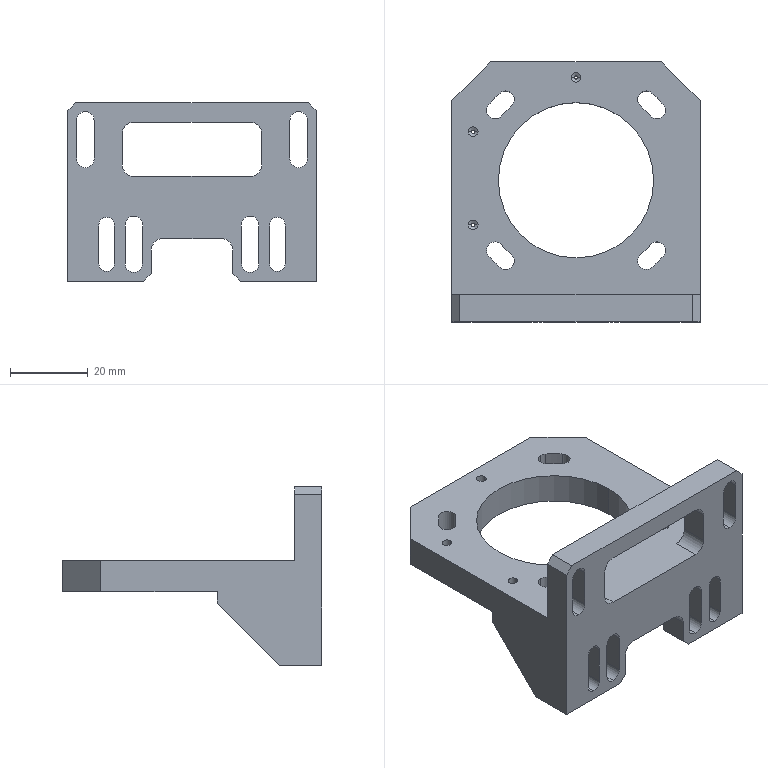NC program | NX | posted with a generic post | part box 64 x 67 x 46 mm
Lines 33235 to 33790 of 33790:
(ZLEVEL_PROFILE_COPY_2_COPY_COPY , TOOL : D6R0.5)
N66426 T05 M6
N66428 G54
N66430 G17 G0 G90 X-34.954 Y33.857 B0. C0. S7000 M3
N66432 G43 Z30. H5
N66434 Z0.929
N66436 G94 G1 Z-0.071 F1000.
N66438 X-34.494 Y33.072
N66440 G3 X-33.972 Y32.776 R0.6
N66442 G1 X-33.751 Y32.778 F3000.
N66444 X-26.233
N66446 X-26.028 Y32.776
N66448 Y32.813 Z-0.106
N66450 Y32.847 Z-0.141
N66452 X-26.233 Y32.849
N66454 X-33.751
N66456 X-33.972 Y32.847
N66458 Y32.884 Z-0.177
N66460 Y32.918 Z-0.212
N66462 X-33.5 Y32.919
N66464 X-26.5
N66466 X-26.028 Y32.917
N66468 Y32.955 Z-0.247
N66470 Y32.988 Z-0.283
N66472 X-26.5 Y32.99
N66474 X-33.5
N66476 X-33.972 Y32.988
N66478 Y33.025 Z-0.318
N66480 Y33.059 Z-0.354
N66482 X-33.5 Y33.061
N66484 X-26.5
N66486 X-26.028 Y33.059
N66488 Y33.096 Z-0.389
N66490 Y33.129 Z-0.424
N66492 X-26.5 Y33.131
N66494 X-33.5
N66496 X-33.972 Y33.13
N66498 Y33.167 Z-0.46
N66500 Y33.2 Z-0.495
N66502 X-33.5 Y33.202
N66504 X-26.5
N66506 X-26.028 Y33.2
N66508 Y33.237 Z-0.53
N66510 Y33.271 Z-0.566
N66512 X-26.5 Y33.273
N66514 X-33.5
N66516 X-33.972 Y33.271
N66518 Y33.308 Z-0.601
N66520 Y33.342 Z-0.636
N66522 X-33.5 Y33.344
N66524 X-26.5
N66526 X-26.028 Y33.342
N66528 Y33.379 Z-0.672
N66530 Y33.412 Z-0.707
N66532 X-26.5 Y33.414
N66534 X-33.5
N66536 X-33.972 Y33.413
N66538 Y33.45 Z-0.742
N66540 Y33.483 Z-0.778
N66542 X-33.5 Y33.485
N66544 X-26.5
N66546 X-26.028 Y33.483
N66548 Y33.52 Z-0.813
N66550 Y33.554 Z-0.849
N66552 X-26.5 Y33.556
N66554 X-33.5
N66556 X-33.972 Y33.554
N66558 Y33.591 Z-0.884
N66560 Y33.625 Z-0.919
N66562 X-33.5 Y33.626
N66564 X-26.5
N66566 X-26.028 Y33.624
N66568 Y33.662 Z-0.955
N66570 Y33.695 Z-0.99
N66572 X-26.5 Y33.697
N66574 X-33.5
N66576 X-33.972 Y33.695
N66578 Y33.732 Z-1.025
N66580 Y33.766 Z-1.061
N66582 X-33.5 Y33.768
N66584 X-26.5
N66586 X-26.028 Y33.766
N66588 Y33.803 Z-1.096
N66590 Y33.837 Z-1.131
N66592 X-26.5 Y33.838
N66594 X-33.5
N66596 X-33.972 Y33.837
N66598 Y33.874 Z-1.167
N66600 Y33.908 Z-1.202
N66602 X-33.5 Y33.909
N66604 X-26.5
N66606 X-26.027 Y33.907
N66608 Y33.945 Z-1.237
N66610 Y33.978 Z-1.273
N66612 X-26.5 Y33.98
N66614 X-33.5
N66616 X-33.972 Y33.978
N66618 Y34.015 Z-1.308
N66620 Y34.049 Z-1.344
N66622 X-33.5 Y34.051
N66624 X-26.5
N66626 X-26.028 Y34.049
N66628 Y34.086 Z-1.379
N66630 Y34.119 Z-1.414
N66632 X-26.5 Y34.121
N66634 X-33.5
N66636 X-33.972 Y34.12
N66638 Y34.157 Z-1.45
N66640 Y34.19 Z-1.485
N66642 X-33.5 Y34.192
N66644 X-26.5
N66646 X-26.028 Y34.19
N66648 Y34.227 Z-1.52
N66650 Y34.261 Z-1.556
N66652 X-26.5 Y34.263
N66654 X-33.5
N66656 X-33.972 Y34.261
N66658 Y34.298 Z-1.591
N66660 Y34.332 Z-1.626
N66662 X-33.5 Y34.333
N66664 X-26.5
N66666 X-26.028 Y34.331
N66668 Y34.369 Z-1.662
N66670 Y34.402 Z-1.697
N66672 X-26.5 Y34.404
N66674 X-33.5
N66676 X-33.972 Y34.403
N66678 Y34.44 Z-1.732
N66680 Y34.473 Z-1.768
N66682 X-33.5 Y34.475
N66684 X-26.5
N66686 X-26.028 Y34.473
N66688 Y34.51 Z-1.803
N66690 Y34.544 Z-1.838
N66692 X-26.5 Y34.546
N66694 X-33.5
N66696 X-33.972 Y34.544
N66698 Y34.581 Z-1.874
N66700 Y34.615 Z-1.909
N66702 X-33.5 Y34.616
N66704 X-26.5
N66706 X-26.028 Y34.614
N66708 Y34.652 Z-1.945
N66710 Y34.685 Z-1.98
N66712 X-26.5 Y34.687
N66714 X-33.5
N66716 X-33.972 Y34.685
N66718 Y34.722 Z-2.015
N66720 Y34.756 Z-2.051
N66722 X-33.5 Y34.758
N66724 X-26.5
N66726 X-26.028 Y34.756
N66728 Y34.793 Z-2.086
N66730 Y34.826 Z-2.121
N66732 X-26.5 Y34.828
N66734 X-33.5
N66736 X-33.972 Y34.827
N66738 Y34.864 Z-2.157
N66740 Y34.897 Z-2.192
N66742 X-33.751 Y34.899
N66744 X-26.233
N66746 X-26.028 Y34.897
N66748 X-26.03 Y34.934 Z-2.227
N66750 X-26.032 Y34.968 Z-2.263
N66752 X-26.233 Y34.97
N66754 X-33.751
N66756 X-33.968 Y34.968
N66758 X-33.909 Y35.028 Z-2.322
N66760 X-26.233 Y35.029
N66762 X-26.087 Y35.028
N66764 X-26.142 Y35.088 Z-2.381
N66766 X-33.849
N66768 X-33.79 Y35.147 Z-2.441
N66770 X-26.196
N66772 G3 X-25.677 Y35.447 R0.6
N66774 G1 X-25.206 Y36.262
N66776 Z-1.441
N66778 G0 Z30.
N66780 X-25.046 Y-33.851
N66782 Z0.929
N66784 G1 Z-0.071 F1000.
N66786 X-25.506 Y-33.071
N66788 G3 X-26.028 Y-32.776 R0.6
N66790 G1 X-26.233 Y-32.778 F3000.
N66792 X-33.751
N66794 X-33.972 Y-32.776
N66796 Y-32.813 Z-0.106
N66798 Y-32.847 Z-0.141
N66800 X-33.751 Y-32.849
N66802 X-26.233
N66804 X-26.028 Y-32.847
N66806 Y-32.884 Z-0.177
N66808 Y-32.917 Z-0.212
N66810 X-26.5 Y-32.919
N66812 X-33.5
N66814 X-33.972 Y-32.918
N66816 Y-32.955 Z-0.247
N66818 Y-32.988 Z-0.283
N66820 X-33.5 Y-32.99
N66822 X-26.5
N66824 X-26.028 Y-32.988
N66826 Y-33.025 Z-0.318
N66828 Y-33.059 Z-0.354
N66830 X-26.5 Y-33.061
N66832 X-33.5
N66834 X-33.972 Y-33.059
N66836 Y-33.096 Z-0.389
N66838 Y-33.13 Z-0.424
N66840 X-33.5 Y-33.131
N66842 X-26.5
N66844 X-26.028 Y-33.129
N66846 Y-33.167 Z-0.46
N66848 Y-33.2 Z-0.495
N66850 X-26.5 Y-33.202
N66852 X-33.5
N66854 X-33.972 Y-33.2
N66856 Y-33.237 Z-0.53
N66858 Y-33.271 Z-0.566
N66860 X-33.5 Y-33.273
N66862 X-26.5
N66864 X-26.028 Y-33.271
N66866 Y-33.308 Z-0.601
N66868 Y-33.342 Z-0.636
N66870 X-26.5 Y-33.344
N66872 X-33.5
N66874 X-33.972 Y-33.342
N66876 Y-33.379 Z-0.672
N66878 Y-33.413 Z-0.707
N66880 X-33.5 Y-33.414
N66882 X-26.5
N66884 X-26.028 Y-33.412
N66886 Y-33.45 Z-0.742
N66888 Y-33.483 Z-0.778
N66890 X-26.5 Y-33.485
N66892 X-33.5
N66894 X-33.972 Y-33.483
N66896 Y-33.52 Z-0.813
N66898 Y-33.554 Z-0.849
N66900 X-33.5 Y-33.556
N66902 X-26.5
N66904 X-26.028 Y-33.554
N66906 Y-33.591 Z-0.884
N66908 Y-33.624 Z-0.919
N66910 X-26.5 Y-33.626
N66912 X-33.5
N66914 X-33.972 Y-33.625
N66916 Y-33.662 Z-0.955
N66918 Y-33.695 Z-0.99
N66920 X-33.5 Y-33.697
N66922 X-26.5
N66924 X-26.028 Y-33.695
N66926 Y-33.732 Z-1.025
N66928 Y-33.766 Z-1.061
N66930 X-26.5 Y-33.768
N66932 X-33.5
N66934 X-33.972 Y-33.766
N66936 Y-33.803 Z-1.096
N66938 Y-33.837 Z-1.131
N66940 X-33.5 Y-33.838
N66942 X-26.5
N66944 X-26.028 Y-33.837
N66946 X-26.027 Y-33.874 Z-1.167
N66948 Y-33.907 Z-1.202
N66950 X-26.5 Y-33.909
N66952 X-33.5
N66954 X-33.972 Y-33.908
N66956 Y-33.945 Z-1.237
N66958 Y-33.978 Z-1.273
N66960 X-33.5 Y-33.98
N66962 X-26.5
N66964 X-26.027 Y-33.978
N66966 X-26.028 Y-34.015 Z-1.308
N66968 Y-34.049 Z-1.344
N66970 X-26.5 Y-34.051
N66972 X-33.5
N66974 X-33.972 Y-34.049
N66976 Y-34.086 Z-1.379
N66978 Y-34.12 Z-1.414
N66980 X-33.5 Y-34.121
N66982 X-26.5
N66984 X-26.028 Y-34.119
N66986 Y-34.157 Z-1.45
N66988 Y-34.19 Z-1.485
N66990 X-26.5 Y-34.192
N66992 X-33.5
N66994 X-33.972 Y-34.19
N66996 Y-34.227 Z-1.52
N66998 Y-34.261 Z-1.556
N67000 X-33.5 Y-34.263
N67002 X-26.5
N67004 X-26.028 Y-34.261
N67006 Y-34.298 Z-1.591
N67008 Y-34.331 Z-1.626
N67010 X-26.5 Y-34.333
N67012 X-33.5
N67014 X-33.972 Y-34.332
N67016 Y-34.369 Z-1.662
N67018 Y-34.403 Z-1.697
N67020 X-33.5 Y-34.404
N67022 X-26.5
N67024 X-26.028 Y-34.402
N67026 Y-34.44 Z-1.732
N67028 Y-34.473 Z-1.768
N67030 X-26.5 Y-34.475
N67032 X-33.5
N67034 X-33.972 Y-34.473
N67036 Y-34.51 Z-1.803
N67038 Y-34.544 Z-1.838
N67040 X-33.5 Y-34.546
N67042 X-26.5
N67044 X-26.028 Y-34.544
N67046 Y-34.581 Z-1.874
N67048 Y-34.614 Z-1.909
N67050 X-26.5 Y-34.616
N67052 X-33.5
N67054 X-33.972 Y-34.615
N67056 Y-34.652 Z-1.945
N67058 Y-34.685 Z-1.98
N67060 X-33.5 Y-34.687
N67062 X-26.5
N67064 X-26.028 Y-34.685
N67066 Y-34.722 Z-2.015
N67068 Y-34.756 Z-2.051
N67070 X-26.5 Y-34.758
N67072 X-33.5
N67074 X-33.972 Y-34.756
N67076 Y-34.793 Z-2.086
N67078 Y-34.827 Z-2.121
N67080 X-33.5 Y-34.828
N67082 X-26.5
N67084 X-26.028 Y-34.826
N67086 Y-34.864 Z-2.157
N67088 Y-34.897 Z-2.192
N67090 X-26.233 Y-34.899
N67092 X-33.751
N67094 X-33.972 Y-34.897
N67096 X-33.97 Y-34.934 Z-2.227
N67098 X-33.968 Y-34.968 Z-2.263
N67100 X-33.751 Y-34.97
N67102 X-26.233
N67104 X-26.032 Y-34.968
N67106 X-26.087 Y-35.028 Z-2.322
N67108 X-26.233 Y-35.029
N67110 X-33.909 Y-35.028
N67112 X-33.849 Y-35.088 Z-2.381
N67114 X-26.142
N67116 X-26.197 Y-35.147 Z-2.441
N67118 X-33.79
N67120 G3 X-34.309 Y-35.447 R0.6
N67122 G1 X-34.782 Y-36.265
N67124 Z-1.441
N67126 G0 Z30.
N67128 M5
(PLANAR_MILL_COPY , TOOL : D6A45)
N67130 T07 M6
N67132 G54
N67134 G17 G0 G90 X-34.9 Y-0.866 B0. C0. S7500 M3
N67136 G43 Z30. H7
N67138 Z0.5
N67140 G94 G1 Z-1. F1250.
N67142 G3 X-34.4 Y0. R1.
N67144 G1 Y32.
N67146 G2 X-33.5 Y32.9 R0.9
N67148 G1 X-26.5
N67150 G2 X-25.6 Y32. R0.9
N67152 G1 Y-32.
N67154 G2 X-26.5 Y-32.9 R0.9
N67156 G1 X-33.5
N67158 G2 X-34.4 Y-32. R0.9
N67160 G1 Y0.
N67162 G3 X-34.9 Y0.866 R1.
N67164 G1 Z0.5
N67166 G0 Z30.
(PLANAR_MILL_COPY_COPY , TOOL : D6A45)
N67168 X-17.458 Y-18.638
N67170 Z-18.5
N67172 G1 Z-20.
N67174 X-17.677 Y-19.452
N67176 G3 X-17.418 Y-20.418 R1.
N67178 X-15.944 Y-21.792 R28.875
N67180 X-14.11 Y-21.664 R1.3
N67182 X-14.238 Y-19.83 R1.3
N67184 G2 X-16.83 Y-17.238 R26.275
N67186 G3 X-18.664 Y-17.11 R1.3
N67188 X-18.792 Y-18.944 R1.3
N67190 X-17.418 Y-20.418 R28.875
N67192 X-16.452 Y-20.677 R1.
N67194 G1 X-15.638 Y-20.458
N67196 Z-18.5
N67198 G0 Z30.
N67200 X1.703 Y-17.853
N67202 Z-18.5
N67204 G1 Z-20.
N67206 X2.134 Y-18.6
N67208 G3 X3. Y-19.1 R1.
N67210 X22.1 Y0. R19.1
N67212 X3. Y-19.1 R-19.1
N67214 X3.866 Y-18.6 R1.
N67216 G1 X4.297 Y-17.853
N67218 Z-18.5
N67220 G0 Z30.
N67222 X-22.408 Y34.313
N67224 Z-18.5
N67226 G1 Z-20.
N67228 X-22.857 Y33.865
N67230 G3 X-23.118 Y32.9 R1.
N67232 G1 X23.459
N67234 G2 X24.166 Y32.607 R1.
N67236 G1 X34.107 Y22.666
N67238 G2 X34.4 Y21.959 R1.
N67240 G1 Y-21.959
N67242 G2 X34.107 Y-22.666 R1.
N67244 G1 X24.166 Y-32.607
N67246 G2 X23.459 Y-32.9 R1.
N67248 G1 X-23.118
N67250 G3 X-22.857 Y-33.865 R1.
N67252 G1 X-22.408 Y-34.313
N67254 Z-18.5
N67256 G0 Z30.
N67258 X21.638 Y-20.458
N67260 Z-18.5
N67262 G1 Z-20.
N67264 X22.452 Y-20.677
N67266 G3 X23.418 Y-20.418 R1.
N67268 X24.792 Y-18.944 R28.875
N67270 X24.664 Y-17.11 R1.3
N67272 X22.83 Y-17.238 R1.3
N67274 G2 X20.238 Y-19.83 R26.275
N67276 G3 X20.11 Y-21.664 R1.3
N67278 X21.944 Y-21.792 R1.3
N67280 X23.418 Y-20.418 R28.875
N67282 X23.677 Y-19.452 R1.
N67284 G1 X23.458 Y-18.638
N67286 Z-18.5
N67288 G0 Z30.
N67290 X29.2 Y-0.198
N67292 Z-18.5
N67294 G1 X29.352 Y-0.35 Z-18.558
N67296 X29.648 Z-18.637
N67298 X29.85 Y-0.148 Z-18.713
N67300 Y0.148 Z-18.793
N67302 X29.648 Y0.35 Z-18.869
N67304 X29.352 Z-18.949
N67306 X29.15 Y0.148 Z-19.025
N67308 Y-0.148 Z-19.105
N67310 X29.352 Y-0.35 Z-19.181
N67312 X29.648 Z-19.26
N67314 X29.85 Y-0.148 Z-19.337
N67316 Y0.148 Z-19.416
N67318 X29.648 Y0.35 Z-19.493
N67320 X29.352 Z-19.572
N67322 X29.15 Y0.148 Z-19.649
N67324 Y-0.148 Z-19.728
N67326 X29.352 Y-0.35 Z-19.804
N67328 X29.648 Z-19.884
N67330 X29.85 Y-0.148 Z-19.96
N67332 Y0. Z-20.
N67334 G3 X29.5 Y0.35 R0.35
N67336 X29.85 Y0. R-0.35
N67338 X29.4 Y-0.217 R0.5
N67340 G1 Z-18.5
N67342 G0 Z30.
N67344 X23.458 Y18.638
N67346 Z-18.5
N67348 G1 Z-20.
N67350 X23.677 Y19.452
N67352 G3 X23.418 Y20.418 R1.
N67354 X21.944 Y21.792 R28.875
N67356 X20.11 Y21.664 R1.3
N67358 X20.238 Y19.83 R1.3
N67360 G2 X22.83 Y17.238 R26.275
N67362 G3 X24.664 Y17.11 R1.3
N67364 X24.792 Y18.944 R1.3
N67366 X23.418 Y20.418 R28.875
N67368 X22.452 Y20.677 R1.
N67370 G1 X21.638 Y20.458
N67372 Z-18.5
N67374 G0 Z30.
N67376 X15.698 Y26.2
N67378 Z-18.5
N67380 G1 X15.85 Y26.352 Z-18.558
N67382 Y26.648 Z-18.637
N67384 X15.648 Y26.85 Z-18.713
N67386 X15.352 Z-18.793
N67388 X15.15 Y26.648 Z-18.869
N67390 Y26.352 Z-18.949
N67392 X15.352 Y26.15 Z-19.025
N67394 X15.648 Z-19.105
N67396 X15.85 Y26.352 Z-19.181
N67398 Y26.648 Z-19.26
N67400 X15.648 Y26.85 Z-19.337
N67402 X15.352 Z-19.416
N67404 X15.15 Y26.648 Z-19.493
N67406 Y26.352 Z-19.572
N67408 X15.352 Y26.15 Z-19.649
N67410 X15.648 Z-19.728
N67412 X15.85 Y26.352 Z-19.804
N67414 Y26.648 Z-19.884
N67416 X15.648 Y26.85 Z-19.96
N67418 X15.5 Z-20.
N67420 G3 X15.15 Y26.5 R0.35
N67422 X15.5 Y26.85 R-0.35
N67424 X15.717 Y26.4 R0.5
N67426 G1 Z-18.5
N67428 G0 Z30.
N67430 X-8.302 Y26.2
N67432 Z-18.5
N67434 G1 X-8.15 Y26.352 Z-18.558
N67436 Y26.648 Z-18.637
N67438 X-8.352 Y26.85 Z-18.713
N67440 X-8.648 Z-18.793
N67442 X-8.85 Y26.648 Z-18.869
N67444 Y26.352 Z-18.949
N67446 X-8.648 Y26.15 Z-19.025
N67448 X-8.352 Z-19.105
N67450 X-8.15 Y26.352 Z-19.181
N67452 Y26.648 Z-19.26
N67454 X-8.352 Y26.85 Z-19.337
N67456 X-8.648 Z-19.416
N67458 X-8.85 Y26.648 Z-19.493
N67460 Y26.352 Z-19.572
N67462 X-8.648 Y26.15 Z-19.649
N67464 X-8.352 Z-19.728
N67466 X-8.15 Y26.352 Z-19.804
N67468 Y26.648 Z-19.884
N67470 X-8.352 Y26.85 Z-19.96
N67472 X-8.5 Z-20.
N67474 G3 X-8.85 Y26.5 R0.35
N67476 X-8.5 Y26.85 R-0.35
N67478 X-8.283 Y26.4 R0.5
N67480 G1 Z-18.5
N67482 G0 Z30.
N67484 X-15.638 Y20.458
N67486 Z-18.5
N67488 G1 Z-20.
N67490 X-16.452 Y20.677
N67492 G3 X-17.418 Y20.418 R1.
N67494 X-18.792 Y18.944 R28.875
N67496 X-18.664 Y17.11 R1.3
N67498 X-16.83 Y17.238 R1.3
N67500 G2 X-14.238 Y19.83 R26.275
N67502 G3 X-14.11 Y21.664 R1.3
N67504 X-15.944 Y21.792 R1.3
N67506 X-17.418 Y20.418 R28.875
N67508 X-17.677 Y19.452 R1.
N67510 G1 X-17.458 Y18.638
N67512 Z-18.5
N67514 G0 Z30.
N67516 M5
N67518 M2